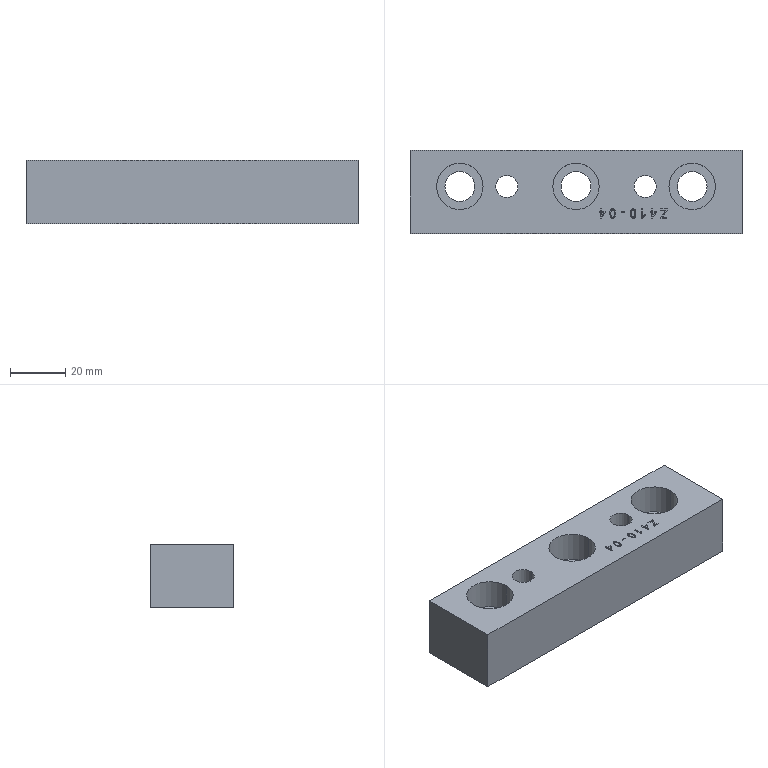Part | Creo | 1 solid | 129 faces | box 120 x 30 x 23 mm | volume 69871 mm3 | plane 61 | other 51 | cylinder 17 | commonest cylinder face diameters 10.8 x6 16.8 x6 8 x4 45.582 x1